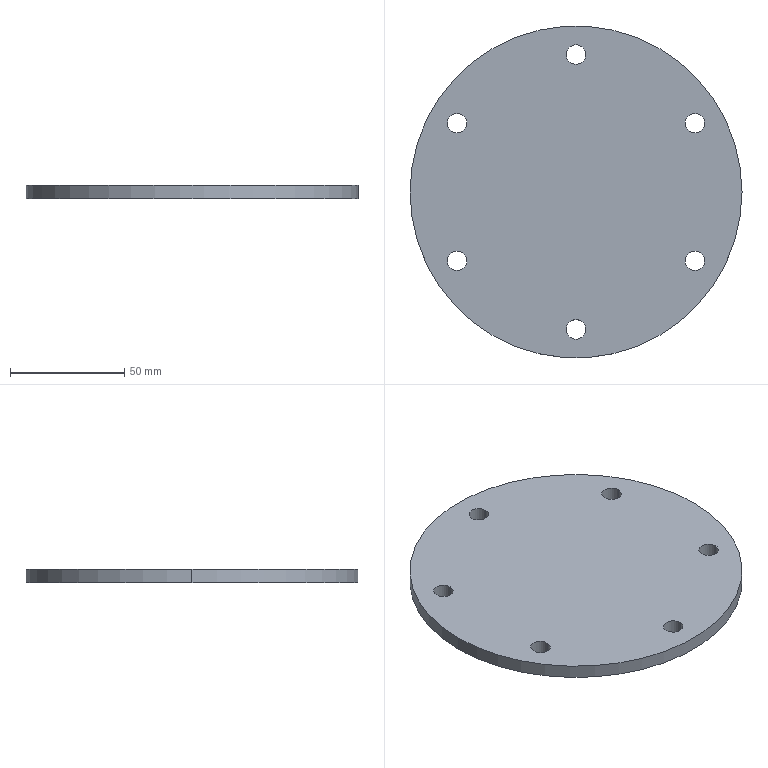Part | SolidWorks | features Extrusion 1 | 1 solid | 16 faces | box 145 x 145 x 6 mm | volume 97035 mm3 | cylinder 14 | plane 2 | commonest cylinder face diameters 8.5 x12 145 x2
STEP:
#1=CARTESIAN_POINT('',(-56.212,30.,6.));
#2=VERTEX_POINT('',#1);
#3=CARTESIAN_POINT('',(-47.712,30.,6.));
#4=VERTEX_POINT('',#3);
#5=CARTESIAN_POINT('',(-51.962,30.,6.));
#6=DIRECTION('',(0.,0.,1.));
#7=DIRECTION('',(1.,0.,0.));
#8=AXIS2_PLACEMENT_3D('',#5,#6,#7);
#9=CIRCLE('',#8,4.25);
#10=EDGE_CURVE('',#2,#4,#9,.T.);
#11=ORIENTED_EDGE('',*,*,#10,.T.);
#12=CARTESIAN_POINT('',(-47.712,30.,0.));
#13=VERTEX_POINT('',#12);
#14=CARTESIAN_POINT('',(-47.712,30.,6.));
#15=DIRECTION('',(0.,0.,-1.));
#16=VECTOR('',#15,1000.);
#17=LINE('',#14,#16);
#18=EDGE_CURVE('',#4,#13,#17,.T.);
#19=ORIENTED_EDGE('',*,*,#18,.T.);
#20=CARTESIAN_POINT('',(-56.212,30.,0.));
#21=VERTEX_POINT('',#20);
#22=CARTESIAN_POINT('',(-51.962,30.,0.));
#23=DIRECTION('',(0.,0.,1.));
#24=DIRECTION('',(1.,0.,0.));
#25=AXIS2_PLACEMENT_3D('',#22,#23,#24);
#26=CIRCLE('',#25,4.25);
#27=EDGE_CURVE('',#21,#13,#26,.T.);
#28=ORIENTED_EDGE('',*,*,#27,.F.);
#29=CARTESIAN_POINT('',(-56.212,30.,6.));
#30=DIRECTION('',(0.,0.,-1.));
#31=VECTOR('',#30,1000.);
#32=LINE('',#29,#31);
#33=EDGE_CURVE('',#2,#21,#32,.T.);
#34=ORIENTED_EDGE('',*,*,#33,.F.);
#35=EDGE_LOOP('',(#11,#19,#28,#34));
#36=FACE_OUTER_BOUND('',#35,.T.);
#37=CARTESIAN_POINT('',(-51.962,30.,6.));
#38=DIRECTION('',(0.,0.,-1.));
#39=DIRECTION('',(-1.,0.,0.));
#40=AXIS2_PLACEMENT_3D('',#37,#38,#39);
#41=CYLINDRICAL_SURFACE('',#40,4.25);
#42=ADVANCED_FACE('',(#36),#41,.F.);
#43=CARTESIAN_POINT('',(-56.212,-30.,6.));
#44=VERTEX_POINT('',#43);
#45=CARTESIAN_POINT('',(-47.712,-30.,6.));
#46=VERTEX_POINT('',#45);
#47=CARTESIAN_POINT('',(-51.962,-30.,6.));
#48=DIRECTION('',(0.,0.,1.));
#49=DIRECTION('',(1.,0.,0.));
#50=AXIS2_PLACEMENT_3D('',#47,#48,#49);
#51=CIRCLE('',#50,4.25);
#52=EDGE_CURVE('',#44,#46,#51,.T.);
#53=ORIENTED_EDGE('',*,*,#52,.T.);
#54=CARTESIAN_POINT('',(-47.712,-30.,0.));
#55=VERTEX_POINT('',#54);
#56=CARTESIAN_POINT('',(-47.712,-30.,6.));
#57=DIRECTION('',(0.,0.,-1.));
#58=VECTOR('',#57,1000.);
#59=LINE('',#56,#58);
#60=EDGE_CURVE('',#46,#55,#59,.T.);
#61=ORIENTED_EDGE('',*,*,#60,.T.);
#62=CARTESIAN_POINT('',(-56.212,-30.,0.));
#63=VERTEX_POINT('',#62);
#64=CARTESIAN_POINT('',(-51.962,-30.,0.));
#65=DIRECTION('',(0.,0.,1.));
#66=DIRECTION('',(1.,0.,0.));
#67=AXIS2_PLACEMENT_3D('',#64,#65,#66);
#68=CIRCLE('',#67,4.25);
#69=EDGE_CURVE('',#63,#55,#68,.T.);
#70=ORIENTED_EDGE('',*,*,#69,.F.);
#71=CARTESIAN_POINT('',(-56.212,-30.,6.));
#72=DIRECTION('',(0.,0.,-1.));
#73=VECTOR('',#72,1000.);
#74=LINE('',#71,#73);
#75=EDGE_CURVE('',#44,#63,#74,.T.);
#76=ORIENTED_EDGE('',*,*,#75,.F.);
#77=EDGE_LOOP('',(#53,#61,#70,#76));
#78=FACE_OUTER_BOUND('',#77,.T.);
#79=CARTESIAN_POINT('',(-51.962,-30.,6.));
#80=DIRECTION('',(0.,0.,-1.));
#81=DIRECTION('',(-1.,0.,0.));
#82=AXIS2_PLACEMENT_3D('',#79,#80,#81);
#83=CYLINDRICAL_SURFACE('',#82,4.25);
#84=ADVANCED_FACE('',(#78),#83,.F.);
#85=CARTESIAN_POINT('',(-4.25,-60.,6.));
#86=VERTEX_POINT('',#85);
#87=CARTESIAN_POINT('',(4.25,-60.,6.));
#88=VERTEX_POINT('',#87);
#89=CARTESIAN_POINT('',(0.,-60.,6.));
#90=DIRECTION('',(0.,0.,1.));
#91=DIRECTION('',(1.,0.,0.));
#92=AXIS2_PLACEMENT_3D('',#89,#90,#91);
#93=CIRCLE('',#92,4.25);
#94=EDGE_CURVE('',#86,#88,#93,.T.);
#95=ORIENTED_EDGE('',*,*,#94,.T.);
#96=CARTESIAN_POINT('',(4.25,-60.,0.));
#97=VERTEX_POINT('',#96);
#98=CARTESIAN_POINT('',(4.25,-60.,6.));
#99=DIRECTION('',(0.,0.,-1.));
#100=VECTOR('',#99,1000.);
#101=LINE('',#98,#100);
#102=EDGE_CURVE('',#88,#97,#101,.T.);
#103=ORIENTED_EDGE('',*,*,#102,.T.);
#104=CARTESIAN_POINT('',(-4.25,-60.,0.));
#105=VERTEX_POINT('',#104);
#106=CARTESIAN_POINT('',(0.,-60.,0.));
#107=DIRECTION('',(0.,0.,1.));
#108=DIRECTION('',(1.,0.,0.));
#109=AXIS2_PLACEMENT_3D('',#106,#107,#108);
#110=CIRCLE('',#109,4.25);
#111=EDGE_CURVE('',#105,#97,#110,.T.);
#112=ORIENTED_EDGE('',*,*,#111,.F.);
#113=CARTESIAN_POINT('',(-4.25,-60.,6.));
#114=DIRECTION('',(0.,0.,-1.));
#115=VECTOR('',#114,1000.);
#116=LINE('',#113,#115);
#117=EDGE_CURVE('',#86,#105,#116,.T.);
#118=ORIENTED_EDGE('',*,*,#117,.F.);
#119=EDGE_LOOP('',(#95,#103,#112,#118));
#120=FACE_OUTER_BOUND('',#119,.T.);
#121=CARTESIAN_POINT('',(0.,-60.,6.));
#122=DIRECTION('',(0.,0.,-1.));
#123=DIRECTION('',(-1.,0.,0.));
#124=AXIS2_PLACEMENT_3D('',#121,#122,#123);
#125=CYLINDRICAL_SURFACE('',#124,4.25);
#126=ADVANCED_FACE('',(#120),#125,.F.);
#127=CARTESIAN_POINT('',(47.712,-30.,6.));
#128=VERTEX_POINT('',#127);
#129=CARTESIAN_POINT('',(56.212,-30.,6.));
#130=VERTEX_POINT('',#129);
#131=CARTESIAN_POINT('',(51.962,-30.,6.));
#132=DIRECTION('',(0.,0.,1.));
#133=DIRECTION('',(1.,0.,0.));
#134=AXIS2_PLACEMENT_3D('',#131,#132,#133);
#135=CIRCLE('',#134,4.25);
#136=EDGE_CURVE('',#128,#130,#135,.T.);
#137=ORIENTED_EDGE('',*,*,#136,.T.);
#138=CARTESIAN_POINT('',(56.212,-30.,0.));
#139=VERTEX_POINT('',#138);
#140=CARTESIAN_POINT('',(56.212,-30.,6.));
#141=DIRECTION('',(0.,0.,-1.));
#142=VECTOR('',#141,1000.);
#143=LINE('',#140,#142);
#144=EDGE_CURVE('',#130,#139,#143,.T.);
#145=ORIENTED_EDGE('',*,*,#144,.T.);
#146=CARTESIAN_POINT('',(47.712,-30.,0.));
#147=VERTEX_POINT('',#146);
#148=CARTESIAN_POINT('',(51.962,-30.,0.));
#149=DIRECTION('',(0.,0.,1.));
#150=DIRECTION('',(1.,0.,0.));
#151=AXIS2_PLACEMENT_3D('',#148,#149,#150);
#152=CIRCLE('',#151,4.25);
#153=EDGE_CURVE('',#147,#139,#152,.T.);
#154=ORIENTED_EDGE('',*,*,#153,.F.);
#155=CARTESIAN_POINT('',(47.712,-30.,6.));
#156=DIRECTION('',(0.,0.,-1.));
#157=VECTOR('',#156,1000.);
#158=LINE('',#155,#157);
#159=EDGE_CURVE('',#128,#147,#158,.T.);
#160=ORIENTED_EDGE('',*,*,#159,.F.);
#161=EDGE_LOOP('',(#137,#145,#154,#160));
#162=FACE_OUTER_BOUND('',#161,.T.);
#163=CARTESIAN_POINT('',(51.962,-30.,6.));
#164=DIRECTION('',(0.,0.,-1.));
#165=DIRECTION('',(-1.,0.,0.));
#166=AXIS2_PLACEMENT_3D('',#163,#164,#165);
#167=CYLINDRICAL_SURFACE('',#166,4.25);
#168=ADVANCED_FACE('',(#162),#167,.F.);
#169=CARTESIAN_POINT('',(47.712,30.,6.));
#170=VERTEX_POINT('',#169);
#171=CARTESIAN_POINT('',(56.212,30.,6.));
#172=VERTEX_POINT('',#171);
#173=CARTESIAN_POINT('',(51.962,30.,6.));
#174=DIRECTION('',(0.,0.,1.));
#175=DIRECTION('',(1.,0.,0.));
#176=AXIS2_PLACEMENT_3D('',#173,#174,#175);
#177=CIRCLE('',#176,4.25);
#178=EDGE_CURVE('',#170,#172,#177,.T.);
#179=ORIENTED_EDGE('',*,*,#178,.T.);
#180=CARTESIAN_POINT('',(56.212,30.,0.));
#181=VERTEX_POINT('',#180);
#182=CARTESIAN_POINT('',(56.212,30.,6.));
#183=DIRECTION('',(0.,0.,-1.));
#184=VECTOR('',#183,1000.);
#185=LINE('',#182,#184);
#186=EDGE_CURVE('',#172,#181,#185,.T.);
#187=ORIENTED_EDGE('',*,*,#186,.T.);
#188=CARTESIAN_POINT('',(47.712,30.,0.));
#189=VERTEX_POINT('',#188);
#190=CARTESIAN_POINT('',(51.962,30.,0.));
#191=DIRECTION('',(0.,0.,1.));
#192=DIRECTION('',(1.,0.,0.));
#193=AXIS2_PLACEMENT_3D('',#190,#191,#192);
#194=CIRCLE('',#193,4.25);
#195=EDGE_CURVE('',#189,#181,#194,.T.);
#196=ORIENTED_EDGE('',*,*,#195,.F.);
#197=CARTESIAN_POINT('',(47.712,30.,6.));
#198=DIRECTION('',(0.,0.,-1.));
#199=VECTOR('',#198,1000.);
#200=LINE('',#197,#199);
#201=EDGE_CURVE('',#170,#189,#200,.T.);
#202=ORIENTED_EDGE('',*,*,#201,.F.);
#203=EDGE_LOOP('',(#179,#187,#196,#202));
#204=FACE_OUTER_BOUND('',#203,.T.);
#205=CARTESIAN_POINT('',(51.962,30.,6.));
#206=DIRECTION('',(0.,0.,-1.));
#207=DIRECTION('',(-1.,0.,0.));
#208=AXIS2_PLACEMENT_3D('',#205,#206,#207);
#209=CYLINDRICAL_SURFACE('',#208,4.25);
#210=ADVANCED_FACE('',(#204),#209,.F.);
#211=CARTESIAN_POINT('',(-4.25,60.,6.));
#212=VERTEX_POINT('',#211);
#213=CARTESIAN_POINT('',(4.25,60.,6.));
#214=VERTEX_POINT('',#213);
#215=CARTESIAN_POINT('',(0.,60.,6.));
#216=DIRECTION('',(0.,0.,1.));
#217=DIRECTION('',(1.,0.,0.));
#218=AXIS2_PLACEMENT_3D('',#215,#216,#217);
#219=CIRCLE('',#218,4.25);
#220=EDGE_CURVE('',#212,#214,#219,.T.);
#221=ORIENTED_EDGE('',*,*,#220,.T.);
#222=CARTESIAN_POINT('',(4.25,60.,0.));
#223=VERTEX_POINT('',#222);
#224=CARTESIAN_POINT('',(4.25,60.,6.));
#225=DIRECTION('',(0.,0.,-1.));
#226=VECTOR('',#225,1000.);
#227=LINE('',#224,#226);
#228=EDGE_CURVE('',#214,#223,#227,.T.);
#229=ORIENTED_EDGE('',*,*,#228,.T.);
#230=CARTESIAN_POINT('',(-4.25,60.,0.));
#231=VERTEX_POINT('',#230);
#232=CARTESIAN_POINT('',(0.,60.,0.));
#233=DIRECTION('',(0.,0.,1.));
#234=DIRECTION('',(1.,0.,0.));
#235=AXIS2_PLACEMENT_3D('',#232,#233,#234);
#236=CIRCLE('',#235,4.25);
#237=EDGE_CURVE('',#231,#223,#236,.T.);
#238=ORIENTED_EDGE('',*,*,#237,.F.);
#239=CARTESIAN_POINT('',(-4.25,60.,6.));
#240=DIRECTION('',(0.,0.,-1.));
#241=VECTOR('',#240,1000.);
#242=LINE('',#239,#241);
#243=EDGE_CURVE('',#212,#231,#242,.T.);
#244=ORIENTED_EDGE('',*,*,#243,.F.);
#245=EDGE_LOOP('',(#221,#229,#238,#244));
#246=FACE_OUTER_BOUND('',#245,.T.);
#247=CARTESIAN_POINT('',(0.,60.,6.));
#248=DIRECTION('',(0.,0.,-1.));
#249=DIRECTION('',(-1.,0.,0.));
#250=AXIS2_PLACEMENT_3D('',#247,#248,#249);
#251=CYLINDRICAL_SURFACE('',#250,4.25);
#252=ADVANCED_FACE('',(#246),#251,.F.);
#253=CARTESIAN_POINT('',(72.5,0.,6.));
#254=VERTEX_POINT('',#253);
#255=CARTESIAN_POINT('',(-72.5,0.,6.));
#256=VERTEX_POINT('',#255);
#257=CARTESIAN_POINT('',(0.,0.,6.));
#258=DIRECTION('',(0.,0.,1.));
#259=DIRECTION('',(1.,0.,0.));
#260=AXIS2_PLACEMENT_3D('',#257,#258,#259);
#261=CIRCLE('',#260,72.5);
#262=EDGE_CURVE('',#254,#256,#261,.T.);
#263=ORIENTED_EDGE('',*,*,#262,.F.);
#264=CARTESIAN_POINT('',(72.5,0.,0.));
#265=VERTEX_POINT('',#264);
#266=CARTESIAN_POINT('',(72.5,0.,6.));
#267=DIRECTION('',(0.,0.,-1.));
#268=VECTOR('',#267,1000.);
#269=LINE('',#266,#268);
#270=EDGE_CURVE('',#254,#265,#269,.T.);
#271=ORIENTED_EDGE('',*,*,#270,.T.);
#272=CARTESIAN_POINT('',(-72.5,0.,0.));
#273=VERTEX_POINT('',#272);
#274=CARTESIAN_POINT('',(0.,0.,0.));
#275=DIRECTION('',(0.,0.,1.));
#276=DIRECTION('',(1.,0.,0.));
#277=AXIS2_PLACEMENT_3D('',#274,#275,#276);
#278=CIRCLE('',#277,72.5);
#279=EDGE_CURVE('',#265,#273,#278,.T.);
#280=ORIENTED_EDGE('',*,*,#279,.T.);
#281=CARTESIAN_POINT('',(-72.5,0.,6.));
#282=DIRECTION('',(0.,0.,-1.));
#283=VECTOR('',#282,1000.);
#284=LINE('',#281,#283);
#285=EDGE_CURVE('',#256,#273,#284,.T.);
#286=ORIENTED_EDGE('',*,*,#285,.F.);
#287=EDGE_LOOP('',(#263,#271,#280,#286));
#288=FACE_OUTER_BOUND('',#287,.T.);
#289=CARTESIAN_POINT('',(0.,0.,6.));
#290=DIRECTION('',(0.,0.,-1.));
#291=DIRECTION('',(-1.,0.,0.));
#292=AXIS2_PLACEMENT_3D('',#289,#290,#291);
#293=CYLINDRICAL_SURFACE('',#292,72.5);
#294=ADVANCED_FACE('',(#288),#293,.T.);
#295=ORIENTED_EDGE('',*,*,#52,.F.);
#296=CARTESIAN_POINT('',(-51.962,-30.,6.));
#297=DIRECTION('',(0.,0.,1.));
#298=DIRECTION('',(1.,0.,0.));
#299=AXIS2_PLACEMENT_3D('',#296,#297,#298);
#300=CIRCLE('',#299,4.25);
#301=EDGE_CURVE('',#46,#44,#300,.T.);
#302=ORIENTED_EDGE('',*,*,#301,.F.);
#303=EDGE_LOOP('',(#295,#302));
#304=FACE_BOUND('',#303,.T.);
#305=ORIENTED_EDGE('',*,*,#136,.F.);
#306=CARTESIAN_POINT('',(51.962,-30.,6.));
#307=DIRECTION('',(0.,0.,1.));
#308=DIRECTION('',(1.,0.,0.));
#309=AXIS2_PLACEMENT_3D('',#306,#307,#308);
#310=CIRCLE('',#309,4.25);
#311=EDGE_CURVE('',#130,#128,#310,.T.);
#312=ORIENTED_EDGE('',*,*,#311,.F.);
#313=EDGE_LOOP('',(#305,#312));
#314=FACE_BOUND('',#313,.T.);
#315=ORIENTED_EDGE('',*,*,#220,.F.);
#316=CARTESIAN_POINT('',(0.,60.,6.));
#317=DIRECTION('',(0.,0.,1.));
#318=DIRECTION('',(1.,0.,0.));
#319=AXIS2_PLACEMENT_3D('',#316,#317,#318);
#320=CIRCLE('',#319,4.25);
#321=EDGE_CURVE('',#214,#212,#320,.T.);
#322=ORIENTED_EDGE('',*,*,#321,.F.);
#323=EDGE_LOOP('',(#315,#322));
#324=FACE_BOUND('',#323,.T.);
#325=CARTESIAN_POINT('',(0.,0.,6.));
#326=DIRECTION('',(0.,0.,1.));
#327=DIRECTION('',(1.,0.,0.));
#328=AXIS2_PLACEMENT_3D('',#325,#326,#327);
#329=CIRCLE('',#328,72.5);
#330=EDGE_CURVE('',#256,#254,#329,.T.);
#331=ORIENTED_EDGE('',*,*,#330,.T.);
#332=ORIENTED_EDGE('',*,*,#262,.T.);
#333=EDGE_LOOP('',(#331,#332));
#334=FACE_OUTER_BOUND('',#333,.T.);
#335=ORIENTED_EDGE('',*,*,#178,.F.);
#336=CARTESIAN_POINT('',(51.962,30.,6.));
#337=DIRECTION('',(0.,0.,1.));
#338=DIRECTION('',(1.,0.,0.));
#339=AXIS2_PLACEMENT_3D('',#336,#337,#338);
#340=CIRCLE('',#339,4.25);
#341=EDGE_CURVE('',#172,#170,#340,.T.);
#342=ORIENTED_EDGE('',*,*,#341,.F.);
#343=EDGE_LOOP('',(#335,#342));
#344=FACE_BOUND('',#343,.T.);
#345=ORIENTED_EDGE('',*,*,#94,.F.);
#346=CARTESIAN_POINT('',(0.,-60.,6.));
#347=DIRECTION('',(0.,0.,1.));
#348=DIRECTION('',(1.,0.,0.));
#349=AXIS2_PLACEMENT_3D('',#346,#347,#348);
#350=CIRCLE('',#349,4.25);
#351=EDGE_CURVE('',#88,#86,#350,.T.);
#352=ORIENTED_EDGE('',*,*,#351,.F.);
#353=EDGE_LOOP('',(#345,#352));
#354=FACE_BOUND('',#353,.T.);
#355=ORIENTED_EDGE('',*,*,#10,.F.);
#356=CARTESIAN_POINT('',(-51.962,30.,6.));
#357=DIRECTION('',(0.,0.,1.));
#358=DIRECTION('',(1.,0.,0.));
#359=AXIS2_PLACEMENT_3D('',#356,#357,#358);
#360=CIRCLE('',#359,4.25);
#361=EDGE_CURVE('',#4,#2,#360,.T.);
#362=ORIENTED_EDGE('',*,*,#361,.F.);
#363=EDGE_LOOP('',(#355,#362));
#364=FACE_BOUND('',#363,.T.);
#365=CARTESIAN_POINT('',(0.,0.,6.));
#366=DIRECTION('',(0.,0.,1.));
#367=DIRECTION('',(1.,0.,0.));
#368=AXIS2_PLACEMENT_3D('',#365,#366,#367);
#369=PLANE('',#368);
#370=ADVANCED_FACE('',(#304,#314,#324,#334,#344,#354,#364),#369,.T.);
#371=CARTESIAN_POINT('',(0.,0.,0.));
#372=DIRECTION('',(0.,0.,1.));
#373=DIRECTION('',(1.,0.,0.));
#374=AXIS2_PLACEMENT_3D('',#371,#372,#373);
#375=CIRCLE('',#374,72.5);
#376=EDGE_CURVE('',#273,#265,#375,.T.);
#377=ORIENTED_EDGE('',*,*,#376,.F.);
#378=ORIENTED_EDGE('',*,*,#279,.F.);
#379=EDGE_LOOP('',(#377,#378));
#380=FACE_OUTER_BOUND('',#379,.T.);
#381=ORIENTED_EDGE('',*,*,#237,.T.);
#382=CARTESIAN_POINT('',(0.,60.,0.));
#383=DIRECTION('',(0.,0.,1.));
#384=DIRECTION('',(1.,0.,0.));
#385=AXIS2_PLACEMENT_3D('',#382,#383,#384);
#386=CIRCLE('',#385,4.25);
#387=EDGE_CURVE('',#223,#231,#386,.T.);
#388=ORIENTED_EDGE('',*,*,#387,.T.);
#389=EDGE_LOOP('',(#381,#388));
#390=FACE_BOUND('',#389,.T.);
#391=ORIENTED_EDGE('',*,*,#195,.T.);
#392=CARTESIAN_POINT('',(51.962,30.,0.));
#393=DIRECTION('',(0.,0.,1.));
#394=DIRECTION('',(1.,0.,0.));
#395=AXIS2_PLACEMENT_3D('',#392,#393,#394);
#396=CIRCLE('',#395,4.25);
#397=EDGE_CURVE('',#181,#189,#396,.T.);
#398=ORIENTED_EDGE('',*,*,#397,.T.);
#399=EDGE_LOOP('',(#391,#398));
#400=FACE_BOUND('',#399,.T.);
#401=ORIENTED_EDGE('',*,*,#153,.T.);
#402=CARTESIAN_POINT('',(51.962,-30.,0.));
#403=DIRECTION('',(0.,0.,1.));
#404=DIRECTION('',(1.,0.,0.));
#405=AXIS2_PLACEMENT_3D('',#402,#403,#404);
#406=CIRCLE('',#405,4.25);
#407=EDGE_CURVE('',#139,#147,#406,.T.);
#408=ORIENTED_EDGE('',*,*,#407,.T.);
#409=EDGE_LOOP('',(#401,#408));
#410=FACE_BOUND('',#409,.T.);
#411=ORIENTED_EDGE('',*,*,#111,.T.);
#412=CARTESIAN_POINT('',(0.,-60.,0.));
#413=DIRECTION('',(0.,0.,1.));
#414=DIRECTION('',(1.,0.,0.));
#415=AXIS2_PLACEMENT_3D('',#412,#413,#414);
#416=CIRCLE('',#415,4.25);
#417=EDGE_CURVE('',#97,#105,#416,.T.);
#418=ORIENTED_EDGE('',*,*,#417,.T.);
#419=EDGE_LOOP('',(#411,#418));
#420=FACE_BOUND('',#419,.T.);
#421=ORIENTED_EDGE('',*,*,#69,.T.);
#422=CARTESIAN_POINT('',(-51.962,-30.,0.));
#423=DIRECTION('',(0.,0.,1.));
#424=DIRECTION('',(1.,0.,0.));
#425=AXIS2_PLACEMENT_3D('',#422,#423,#424);
#426=CIRCLE('',#425,4.25);
#427=EDGE_CURVE('',#55,#63,#426,.T.);
#428=ORIENTED_EDGE('',*,*,#427,.T.);
#429=EDGE_LOOP('',(#421,#428));
#430=FACE_BOUND('',#429,.T.);
#431=ORIENTED_EDGE('',*,*,#27,.T.);
#432=CARTESIAN_POINT('',(-51.962,30.,0.));
#433=DIRECTION('',(0.,0.,1.));
#434=DIRECTION('',(1.,0.,0.));
#435=AXIS2_PLACEMENT_3D('',#432,#433,#434);
#436=CIRCLE('',#435,4.25);
#437=EDGE_CURVE('',#13,#21,#436,.T.);
#438=ORIENTED_EDGE('',*,*,#437,.T.);
#439=EDGE_LOOP('',(#431,#438));
#440=FACE_BOUND('',#439,.T.);
#441=CARTESIAN_POINT('',(0.,0.,0.));
#442=DIRECTION('',(0.,0.,1.));
#443=DIRECTION('',(1.,0.,0.));
#444=AXIS2_PLACEMENT_3D('',#441,#442,#443);
#445=PLANE('',#444);
#446=ADVANCED_FACE('',(#380,#390,#400,#410,#420,#430,#440),#445,.F.);
#447=ORIENTED_EDGE('',*,*,#270,.F.);
#448=ORIENTED_EDGE('',*,*,#330,.F.);
#449=ORIENTED_EDGE('',*,*,#285,.T.);
#450=ORIENTED_EDGE('',*,*,#376,.T.);
#451=EDGE_LOOP('',(#447,#448,#449,#450));
#452=FACE_OUTER_BOUND('',#451,.T.);
#453=CARTESIAN_POINT('',(0.,0.,6.));
#454=DIRECTION('',(0.,0.,-1.));
#455=DIRECTION('',(-1.,0.,0.));
#456=AXIS2_PLACEMENT_3D('',#453,#454,#455);
#457=CYLINDRICAL_SURFACE('',#456,72.5);
#458=ADVANCED_FACE('',(#452),#457,.T.);
#459=ORIENTED_EDGE('',*,*,#228,.F.);
#460=ORIENTED_EDGE('',*,*,#321,.T.);
#461=ORIENTED_EDGE('',*,*,#243,.T.);
#462=ORIENTED_EDGE('',*,*,#387,.F.);
#463=EDGE_LOOP('',(#459,#460,#461,#462));
#464=FACE_OUTER_BOUND('',#463,.T.);
#465=CARTESIAN_POINT('',(0.,60.,6.));
#466=DIRECTION('',(0.,0.,-1.));
#467=DIRECTION('',(-1.,0.,0.));
#468=AXIS2_PLACEMENT_3D('',#465,#466,#467);
#469=CYLINDRICAL_SURFACE('',#468,4.25);
#470=ADVANCED_FACE('',(#464),#469,.F.);
#471=ORIENTED_EDGE('',*,*,#186,.F.);
#472=ORIENTED_EDGE('',*,*,#341,.T.);
#473=ORIENTED_EDGE('',*,*,#201,.T.);
#474=ORIENTED_EDGE('',*,*,#397,.F.);
#475=EDGE_LOOP('',(#471,#472,#473,#474));
#476=FACE_OUTER_BOUND('',#475,.T.);
#477=CARTESIAN_POINT('',(51.962,30.,6.));
#478=DIRECTION('',(0.,0.,-1.));
#479=DIRECTION('',(-1.,0.,0.));
#480=AXIS2_PLACEMENT_3D('',#477,#478,#479);
#481=CYLINDRICAL_SURFACE('',#480,4.25);
#482=ADVANCED_FACE('',(#476),#481,.F.);
#483=ORIENTED_EDGE('',*,*,#144,.F.);
#484=ORIENTED_EDGE('',*,*,#311,.T.);
#485=ORIENTED_EDGE('',*,*,#159,.T.);
#486=ORIENTED_EDGE('',*,*,#407,.F.);
#487=EDGE_LOOP('',(#483,#484,#485,#486));
#488=FACE_OUTER_BOUND('',#487,.T.);
#489=CARTESIAN_POINT('',(51.962,-30.,6.));
#490=DIRECTION('',(0.,0.,-1.));
#491=DIRECTION('',(-1.,0.,0.));
#492=AXIS2_PLACEMENT_3D('',#489,#490,#491);
#493=CYLINDRICAL_SURFACE('',#492,4.25);
#494=ADVANCED_FACE('',(#488),#493,.F.);
#495=ORIENTED_EDGE('',*,*,#102,.F.);
#496=ORIENTED_EDGE('',*,*,#351,.T.);
#497=ORIENTED_EDGE('',*,*,#117,.T.);
#498=ORIENTED_EDGE('',*,*,#417,.F.);
#499=EDGE_LOOP('',(#495,#496,#497,#498));
#500=FACE_OUTER_BOUND('',#499,.T.);
#501=CARTESIAN_POINT('',(0.,-60.,6.));
#502=DIRECTION('',(0.,0.,-1.));
#503=DIRECTION('',(-1.,0.,0.));
#504=AXIS2_PLACEMENT_3D('',#501,#502,#503);
#505=CYLINDRICAL_SURFACE('',#504,4.25);
#506=ADVANCED_FACE('',(#500),#505,.F.);
#507=ORIENTED_EDGE('',*,*,#60,.F.);
#508=ORIENTED_EDGE('',*,*,#301,.T.);
#509=ORIENTED_EDGE('',*,*,#75,.T.);
#510=ORIENTED_EDGE('',*,*,#427,.F.);
#511=EDGE_LOOP('',(#507,#508,#509,#510));
#512=FACE_OUTER_BOUND('',#511,.T.);
#513=CARTESIAN_POINT('',(-51.962,-30.,6.));
#514=DIRECTION('',(0.,0.,-1.));
#515=DIRECTION('',(-1.,0.,0.));
#516=AXIS2_PLACEMENT_3D('',#513,#514,#515);
#517=CYLINDRICAL_SURFACE('',#516,4.25);
#518=ADVANCED_FACE('',(#512),#517,.F.);
#519=ORIENTED_EDGE('',*,*,#18,.F.);
#520=ORIENTED_EDGE('',*,*,#361,.T.);
#521=ORIENTED_EDGE('',*,*,#33,.T.);
#522=ORIENTED_EDGE('',*,*,#437,.F.);
#523=EDGE_LOOP('',(#519,#520,#521,#522));
#524=FACE_OUTER_BOUND('',#523,.T.);
#525=CARTESIAN_POINT('',(-51.962,30.,6.));
#526=DIRECTION('',(0.,0.,-1.));
#527=DIRECTION('',(-1.,0.,0.));
#528=AXIS2_PLACEMENT_3D('',#525,#526,#527);
#529=CYLINDRICAL_SURFACE('',#528,4.25);
#530=ADVANCED_FACE('',(#524),#529,.F.);
#531=CLOSED_SHELL('',(#42,#84,#126,#168,#210,#252,#294,#370,#446,#458,#470,#482,#494,#506,#518,#530));
#532=MANIFOLD_SOLID_BREP('',#531);
#533=CARTESIAN_POINT('',(0.,0.,0.));
#534=DIRECTION('',(0.,0.,1.));
#535=DIRECTION('',(1.,0.,0.));
#536=AXIS2_PLACEMENT_3D('',#533,#534,#535);
#537=(LENGTH_UNIT()NAMED_UNIT(*)SI_UNIT(.MILLI.,.METRE.));
#538=UNCERTAINTY_MEASURE_WITH_UNIT(LENGTH_MEASURE(0.00001),#537,'','');
#539=(NAMED_UNIT(*)PLANE_ANGLE_UNIT()SI_UNIT($,.RADIAN.));
#540=(NAMED_UNIT(*)SI_UNIT($,.STERADIAN.)SOLID_ANGLE_UNIT());
#541=(GEOMETRIC_REPRESENTATION_CONTEXT(3)GLOBAL_UNCERTAINTY_ASSIGNED_CONTEXT((#538))GLOBAL_UNIT_ASSIGNED_CONTEXT((#537,#539,#540))REPRESENTATION_CONTEXT('',''));
#542=ADVANCED_BREP_SHAPE_REPRESENTATION('',(#532,#536),#541);